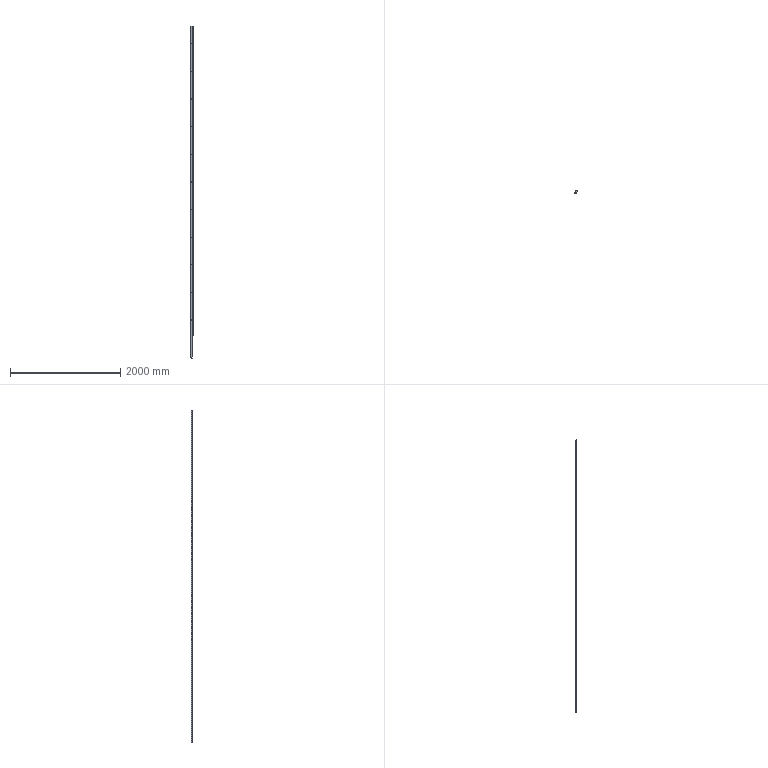Part | STEP file | ASND-0110-5.2 | 1 solid | 60 faces | box 44.772 x 36.1 x 6010 mm | volume 4283109 mm3 | plane 34 | cylinder 26 | commonest cylinder face diameters 4.595 x22 20 x4